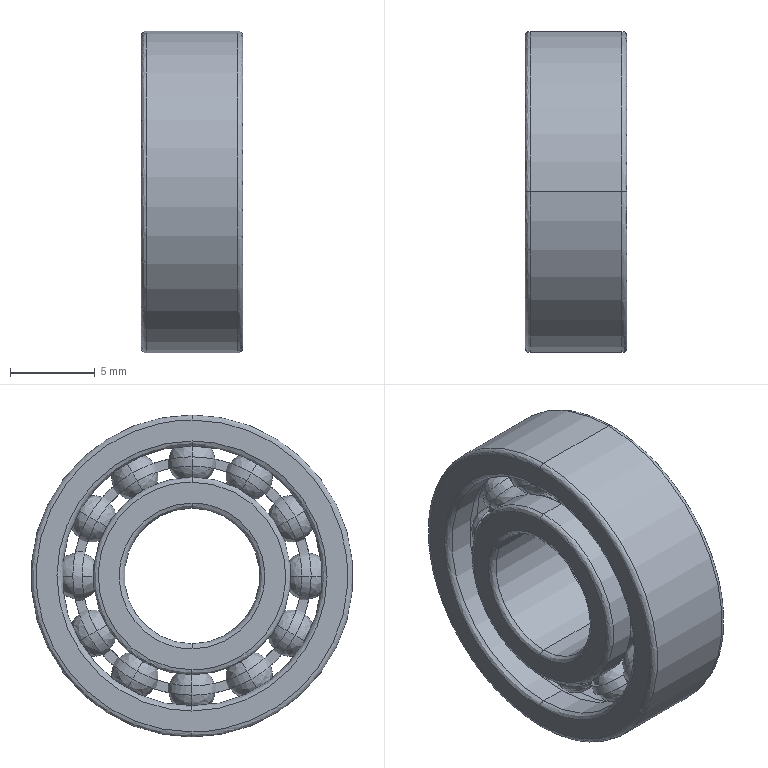Part | SolidWorks | features BaseBody 14 | 14 solids | 159 faces | box 6 x 19 x 19 mm | volume 1020 mm3 | spline 73 | cylinder 58 | plane 28 | commonest cylinder face diameters 12.95 x23 14.05 x23 11.667 x4 15.333 x4 8 x2 19 x2